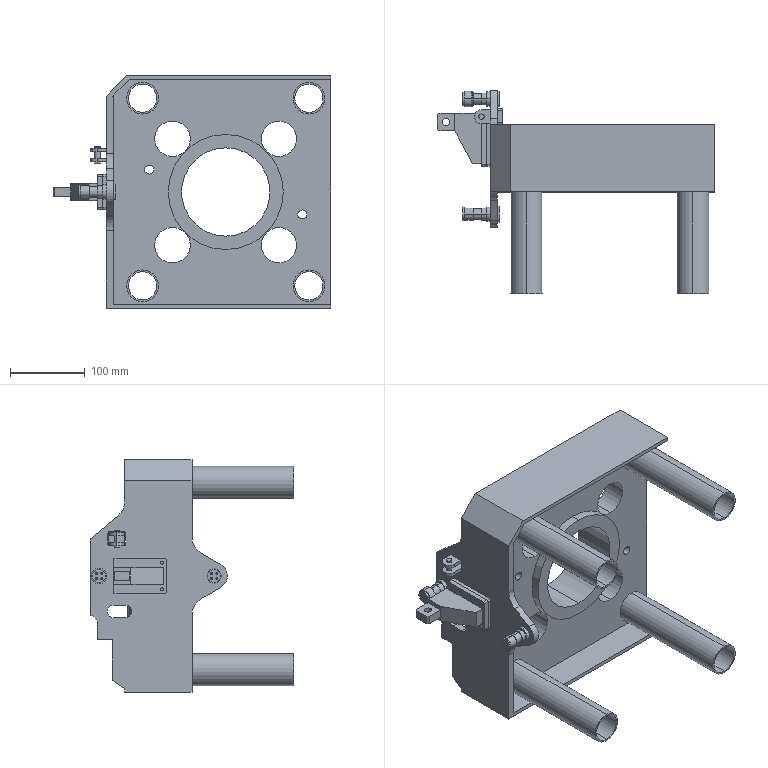Part | SolidWorks | features BaseBody 47, ICE 1, Scale 1 | 35 solids | 676 faces | box 371.182 x 272.09 x 310.892 mm | volume 3352591 mm3 | cylinder 340 | plane 217 | cone 87 | torus 32 | commonest cylinder face diameters 2.484 x48 3.431 x32 3.904 x21 14.196 x20 2.082 x16 3.36 x16